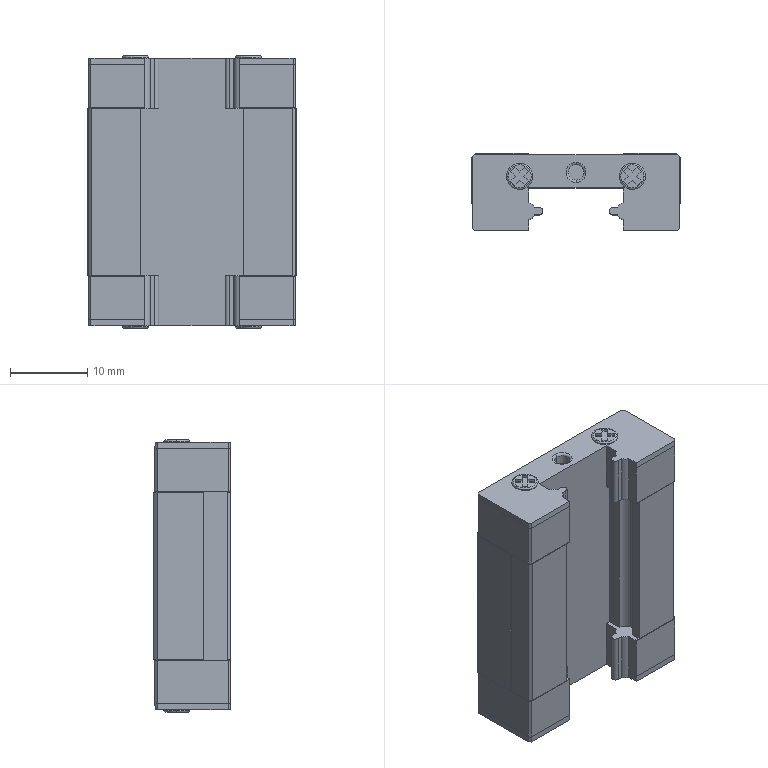Part | STEP file | C-MLGB12 | 1 solid | 229 faces | box 27 x 10 x 35.3 mm | volume 6611 mm3 | plane 164 | cylinder 37 | cone 16 | torus 12 | commonest cylinder face diameters 2.38 x11 2.459 x8 3.4 x8 1 x6 2 x4